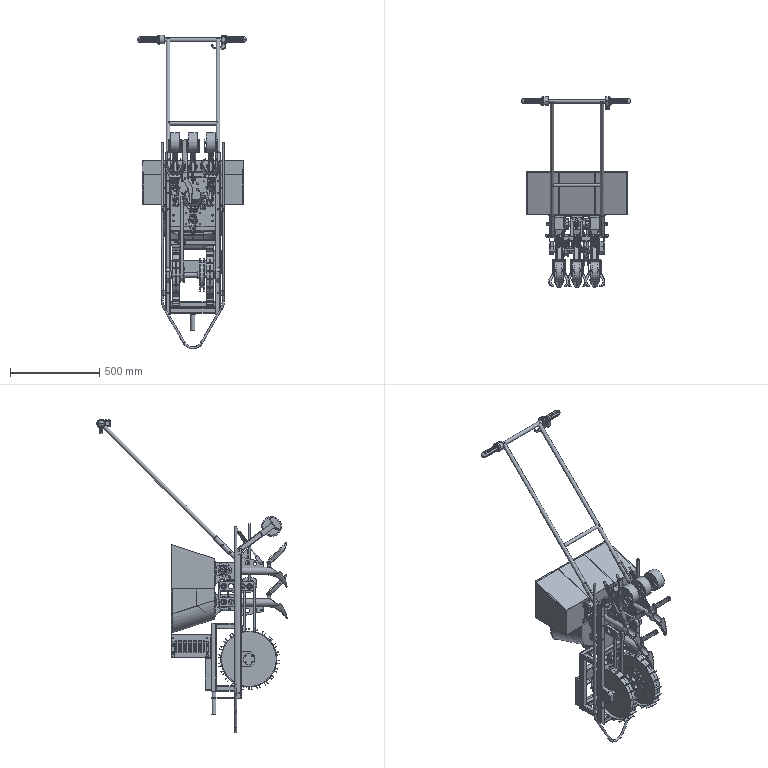Part | NX | features EXTRUDE 104, DATUM_CSYS 73, SKETCH 72, EXTRACT_DATUM_PLANE 44, BREP 35, EXTRACT_BODY 25, UNITE 17, LINKED_FACE 16, BLEND 8, LINKED_BODY 5, SHELL 5, CHAMFER 4, SUBTRACT 4, SWP104 4, INTERSECT 3, DATUM_PLANE 2, Delete Body 2, EXTRACT_STRING 2, Pattern Geometry 2, Container 1, DRAFT 1, Geometry Instance 1, Instance Feature 1, MOVE_FACE 1, Mirror Feature 1, REPLACE_FACE 1 | 247 solids | 5795 faces | volume 13012932 mm3 | plane 2917 | cylinder 2140 | torus 322 | cone 204 | spline 126 | sphere 86 | commonest cylinder face diameters 10 x167 8 x152 2 x106 7.77 x99 30 x92 20 x87